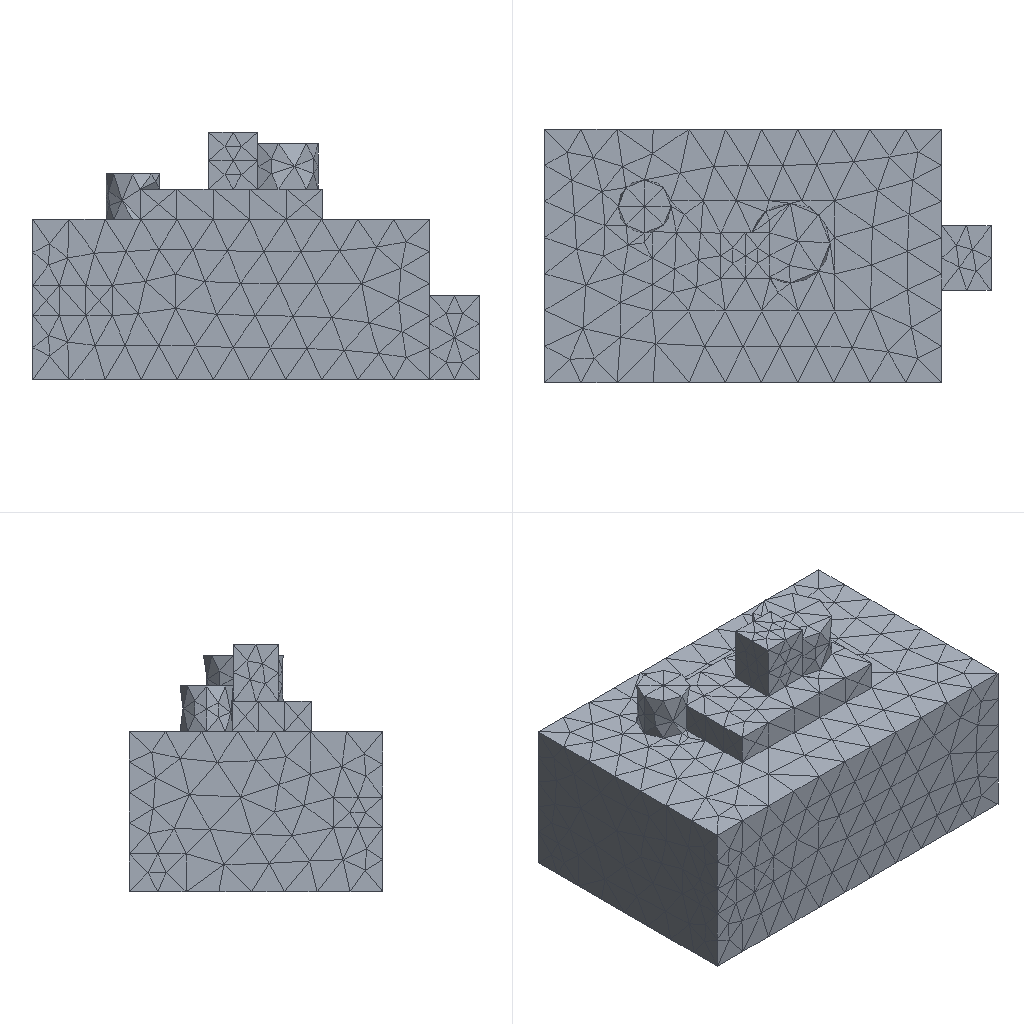Simulation study | ansys mapdl
Set-up summary:
category,name,step,type,value,unit,region
solver,ansys_mapdl
units,mm-N-s-tonne (MPa),,inferred,E=210000 density=
analysis,model,,static
mesh,nodes,,,6885
mesh,elements,,,4274
element_type,SOLID187,,,4274
material,mat 1,,E,210000
material,mat 1,,nu,0.3
load,,model,body load temp,,,all
load,,model,force,"1000 [dir=(0, 0, -1) n=446]",,node list
bc,,model,fixed,"[dofs=UX,UY,UZ n=6800]",,node list
Ansys APDL input file, long lists of numbers shortened:
/COM,ANSYS RELEASE 2026 R1           BUILD 26.1      UP20260202       09:04:29
/PREP7
/NOPR
/TITLE,2
ANTYPE, 0
*IF,_CDRDOFF,EQ,1,THEN     !if solid model was read in
_CDRDOFF=             !reset flag, numoffs already performed
*ELSE              !offset database for the following FE model
NUMOFF,NODE,     6885
NUMOFF,ELEM,     4274
NUMOFF,MAT ,        1
NUMOFF,TYPE,        1
*ENDIF
*SET,_RETURN ,  0.
*SET,_STATUS ,  0.
*SET,_UIQR   ,  446.
*SET,__FLOATPARAMETER__,  6885.
DOF,DELETE
ETBLOCK,        1,        1
(2i9,19a9)
        1      187        0        0        0        0        0        0        0        0        0        0        0        0        0        0        0        0        0        0        0
       -1
NBLOCK,6,SOLID,      6885,      6885
(3i9,6e21.13e3)
        1        0        0 7.0000000000000E+000 6.0000000000000E+000 6.5290000000000E+001
! (6884 more lines like these left out)
N,UNBL,LOC,       -1,
EBLOCK,19,SOLID,      4274,      4274
(19i10)
         1         1         1         1         0         0         0         0        10         0         1      2275       467       182        14      2727       764      2728      2729
! (8547 more lines like these left out)
        -1
MPTEMP,UNBL, 1, 1,  0.    ,
MPDATA,UNBL, 1,EX  ,       1, 1,  210000.000    ,
MPTEMP,UNBL, 1, 1,  0.    ,
MPDATA,UNBL, 1,NUXY,       1, 1, 0.3    ,
MPTEMP,UNBL, 1, 1,  0.    ,
MPDATA,UNBL, 1,PRXY,       1, 1, 0.3    ,
EXTOPT,ATTR,      0,      0,      0
EXTOPT,ESIZE,  0,  0.
EXTOPT,ACLEAR,      0
TREF,  0.
IRLF,  0
BFUNIF,TEMP,_TINY
ACEL,  0.    ,  0.    ,  0.
OMEGA,  0.    ,  0.    ,  0.
DOMEGA,  0.    ,  0.    ,  0.
CGLOC,  0.    ,  0.    ,  0.
CGOMEGA,  0.    ,  0.    ,  0.
DCGOMG,  0.    ,  0.    ,  0.
KUSE,     0
TIME,  0.
ALPHAD,  0.
BETAD,  0.
DMPRAT,  0.
DMPSTR,  0.
CRPLIM, 0.1    ,   0
CRPLIM,  0.    ,   1
NCNV,     0, 1.000000000E+12,     0,  0.    ,  0.
NEQIT,     0
ERESX,DEFA
DBLOCK,      6800
(i9,a6,2(pg16.9))
      387  UX    0.00000000      0.00000000
! (6799 more lines like these left out)
       -1
FBLOCK,       446
(i9,a6,2(pg16.9))
        1  FZ   -2.24215247      0.00000000
! (445 more lines like these left out)
       -1
/GO
FINISH
Results summary:
result,analysis_type_db,,,static,unstated
result,n_sets,,,1,unstated
result,load_steps[0].set,load_step=1,,1,unstated
result,load_steps[0].substep,load_step=1,,1,unstated
result,load_steps[0].time,load_step=1,,1,unstated
result,load_steps[0].freq,load_step=1,,1,unstated
result,load_steps[0].max_usum,load_step=1,,0.0003694,unstated
result,load_steps[0].max_seqv,load_step=1,,5.254,unstated
result,load_steps[0].reaction_sum.FX,load_step=1,,4.54019e-11,unstated
result,load_steps[0].reaction_sum.FY,load_step=1,,-7.85332e-11,unstated
result,load_steps[0].reaction_sum.FZ,load_step=1,,1000,unstated
result,load_steps[0].reaction_sum.MX,load_step=1,,0,unstated
result,load_steps[0].reaction_sum.MY,load_step=1,,0,unstated
result,load_steps[0].reaction_sum.MZ,load_step=1,,0,unstated
result,convergence,,,results present for all listed sets,unstated